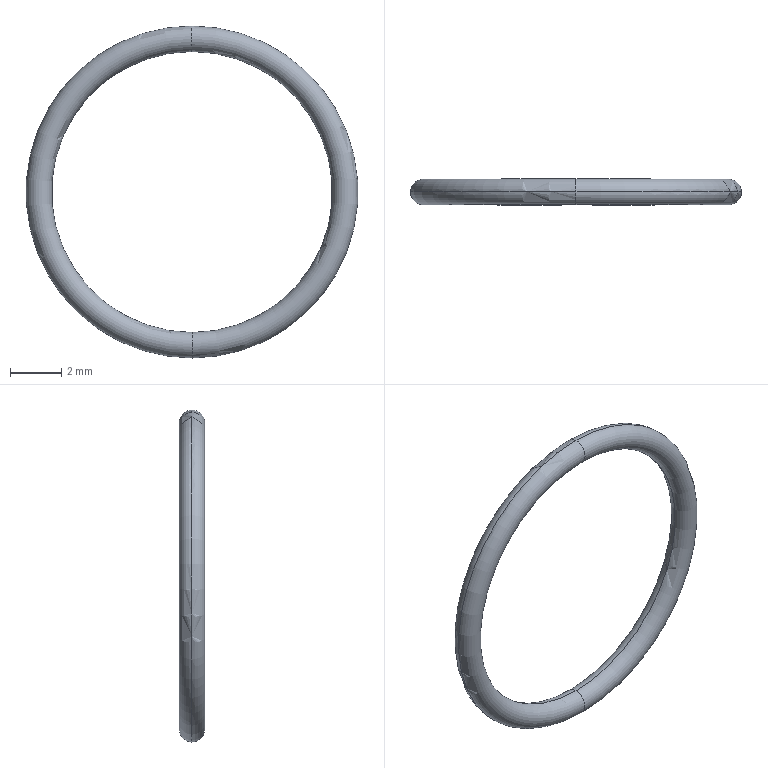Part | NX | features BREP 1 | 1 solid | 4 faces | box 13 x 1 x 13 mm | volume 29.609 mm3 | torus 4
STEP:
#1=CARTESIAN_POINT('',(0.,0.5,-5.5));
#2=VERTEX_POINT('',#1);
#3=CARTESIAN_POINT('',(0.,0.5,-6.5));
#4=VERTEX_POINT('',#3);
#5=CARTESIAN_POINT('',(0.,0.5,-6.));
#6=DIRECTION('',(-1.,0.,0.));
#7=DIRECTION('',(0.,0.,-1.));
#8=AXIS2_PLACEMENT_3D('',#5,#6,#7);
#9=CIRCLE('',#8,0.5);
#10=EDGE_CURVE('',#2,#4,#9,.T.);
#11=ORIENTED_EDGE('',*,*,#10,.T.);
#12=CARTESIAN_POINT('',(0.,0.5,6.5));
#13=VERTEX_POINT('',#12);
#14=CARTESIAN_POINT('',(0.,0.5,0.));
#15=DIRECTION('',(0.,1.,0.));
#16=DIRECTION('',(1.,0.,0.));
#17=AXIS2_PLACEMENT_3D('',#14,#15,#16);
#18=CIRCLE('',#17,6.5);
#19=EDGE_CURVE('',#4,#13,#18,.T.);
#20=ORIENTED_EDGE('',*,*,#19,.T.);
#21=CARTESIAN_POINT('',(0.,1.,6.));
#22=VERTEX_POINT('',#21);
#23=CARTESIAN_POINT('',(0.,0.5,6.));
#24=DIRECTION('',(1.,0.,0.));
#25=DIRECTION('',(0.,0.,-1.));
#26=AXIS2_PLACEMENT_3D('',#23,#24,#25);
#27=CIRCLE('',#26,0.5);
#28=EDGE_CURVE('',#22,#13,#27,.T.);
#29=ORIENTED_EDGE('',*,*,#28,.F.);
#30=CARTESIAN_POINT('',(0.,0.5,5.5));
#31=VERTEX_POINT('',#30);
#32=CARTESIAN_POINT('',(0.,0.5,6.));
#33=DIRECTION('',(-1.,0.,0.));
#34=DIRECTION('',(0.,0.,-1.));
#35=AXIS2_PLACEMENT_3D('',#32,#33,#34);
#36=CIRCLE('',#35,0.5);
#37=EDGE_CURVE('',#22,#31,#36,.T.);
#38=ORIENTED_EDGE('',*,*,#37,.T.);
#39=CARTESIAN_POINT('',(0.,0.5,0.));
#40=DIRECTION('',(0.,1.,0.));
#41=DIRECTION('',(1.,0.,0.));
#42=AXIS2_PLACEMENT_3D('',#39,#40,#41);
#43=CIRCLE('',#42,5.5);
#44=EDGE_CURVE('',#2,#31,#43,.T.);
#45=ORIENTED_EDGE('',*,*,#44,.F.);
#46=EDGE_LOOP('',(#11,#20,#29,#38,#45));
#47=FACE_BOUND('',#46,.T.);
#48=CARTESIAN_POINT('',(0.,0.5,0.));
#49=DIRECTION('',(0.,1.,0.));
#50=DIRECTION('',(0.,0.,1.));
#51=AXIS2_PLACEMENT_3D('',#48,#49,#50);
#52=TOROIDAL_SURFACE('',#51,6.,0.5);
#53=ADVANCED_FACE('',(#47),#52,.T.);
#54=ORIENTED_EDGE('',*,*,#37,.F.);
#55=ORIENTED_EDGE('',*,*,#28,.T.);
#56=CARTESIAN_POINT('',(0.,0.5,0.));
#57=DIRECTION('',(0.,1.,0.));
#58=DIRECTION('',(1.,0.,0.));
#59=AXIS2_PLACEMENT_3D('',#56,#57,#58);
#60=CIRCLE('',#59,6.5);
#61=EDGE_CURVE('',#13,#4,#60,.T.);
#62=ORIENTED_EDGE('',*,*,#61,.T.);
#63=ORIENTED_EDGE('',*,*,#10,.F.);
#64=CARTESIAN_POINT('',(0.,0.5,0.));
#65=DIRECTION('',(0.,1.,0.));
#66=DIRECTION('',(1.,0.,0.));
#67=AXIS2_PLACEMENT_3D('',#64,#65,#66);
#68=CIRCLE('',#67,5.5);
#69=EDGE_CURVE('',#31,#2,#68,.T.);
#70=ORIENTED_EDGE('',*,*,#69,.F.);
#71=EDGE_LOOP('',(#54,#55,#62,#63,#70));
#72=FACE_BOUND('',#71,.T.);
#73=CARTESIAN_POINT('',(0.,0.5,0.));
#74=DIRECTION('',(0.,1.,0.));
#75=DIRECTION('',(0.,0.,-1.));
#76=AXIS2_PLACEMENT_3D('',#73,#74,#75);
#77=TOROIDAL_SURFACE('',#76,6.,0.5);
#78=ADVANCED_FACE('',(#72),#77,.T.);
#79=ORIENTED_EDGE('',*,*,#19,.F.);
#80=CARTESIAN_POINT('',(0.,0.5,-6.));
#81=DIRECTION('',(1.,0.,0.));
#82=DIRECTION('',(0.,0.,-1.));
#83=AXIS2_PLACEMENT_3D('',#80,#81,#82);
#84=CIRCLE('',#83,0.5);
#85=EDGE_CURVE('',#2,#4,#84,.T.);
#86=ORIENTED_EDGE('',*,*,#85,.F.);
#87=ORIENTED_EDGE('',*,*,#44,.T.);
#88=CARTESIAN_POINT('',(0.,0.,6.));
#89=VERTEX_POINT('',#88);
#90=CARTESIAN_POINT('',(0.,0.5,6.));
#91=DIRECTION('',(-1.,0.,0.));
#92=DIRECTION('',(0.,0.,-1.));
#93=AXIS2_PLACEMENT_3D('',#90,#91,#92);
#94=CIRCLE('',#93,0.5);
#95=EDGE_CURVE('',#31,#89,#94,.T.);
#96=ORIENTED_EDGE('',*,*,#95,.T.);
#97=CARTESIAN_POINT('',(0.,0.5,6.));
#98=DIRECTION('',(-1.,0.,0.));
#99=DIRECTION('',(0.,0.,-1.));
#100=AXIS2_PLACEMENT_3D('',#97,#98,#99);
#101=CIRCLE('',#100,0.5);
#102=EDGE_CURVE('',#89,#13,#101,.T.);
#103=ORIENTED_EDGE('',*,*,#102,.T.);
#104=EDGE_LOOP('',(#79,#86,#87,#96,#103));
#105=FACE_BOUND('',#104,.T.);
#106=CARTESIAN_POINT('',(0.,0.5,0.));
#107=DIRECTION('',(0.,1.,0.));
#108=DIRECTION('',(0.,0.,1.));
#109=AXIS2_PLACEMENT_3D('',#106,#107,#108);
#110=TOROIDAL_SURFACE('',#109,6.,0.5);
#111=ADVANCED_FACE('',(#105),#110,.T.);
#112=ORIENTED_EDGE('',*,*,#61,.F.);
#113=ORIENTED_EDGE('',*,*,#102,.F.);
#114=ORIENTED_EDGE('',*,*,#95,.F.);
#115=ORIENTED_EDGE('',*,*,#69,.T.);
#116=ORIENTED_EDGE('',*,*,#85,.T.);
#117=EDGE_LOOP('',(#112,#113,#114,#115,#116));
#118=FACE_BOUND('',#117,.T.);
#119=CARTESIAN_POINT('',(0.,0.5,0.));
#120=DIRECTION('',(0.,1.,0.));
#121=DIRECTION('',(0.,0.,-1.));
#122=AXIS2_PLACEMENT_3D('',#119,#120,#121);
#123=TOROIDAL_SURFACE('',#122,6.,0.5);
#124=ADVANCED_FACE('',(#118),#123,.T.);
#125=CLOSED_SHELL('',(#53,#78,#111,#124));
#126=MANIFOLD_SOLID_BREP('',#125);
#127=(LENGTH_UNIT()NAMED_UNIT(*)SI_UNIT(.MILLI.,.METRE.));
#128=UNCERTAINTY_MEASURE_WITH_UNIT(LENGTH_MEASURE(0.00001),#127,'','');
#129=(NAMED_UNIT(*)PLANE_ANGLE_UNIT()SI_UNIT($,.RADIAN.));
#130=(NAMED_UNIT(*)SI_UNIT($,.STERADIAN.)SOLID_ANGLE_UNIT());
#131=(GEOMETRIC_REPRESENTATION_CONTEXT(3)GLOBAL_UNCERTAINTY_ASSIGNED_CONTEXT((#128))GLOBAL_UNIT_ASSIGNED_CONTEXT((#127,#129,#130))REPRESENTATION_CONTEXT('',''));
#132=ADVANCED_BREP_SHAPE_REPRESENTATION('',(#126),#131);